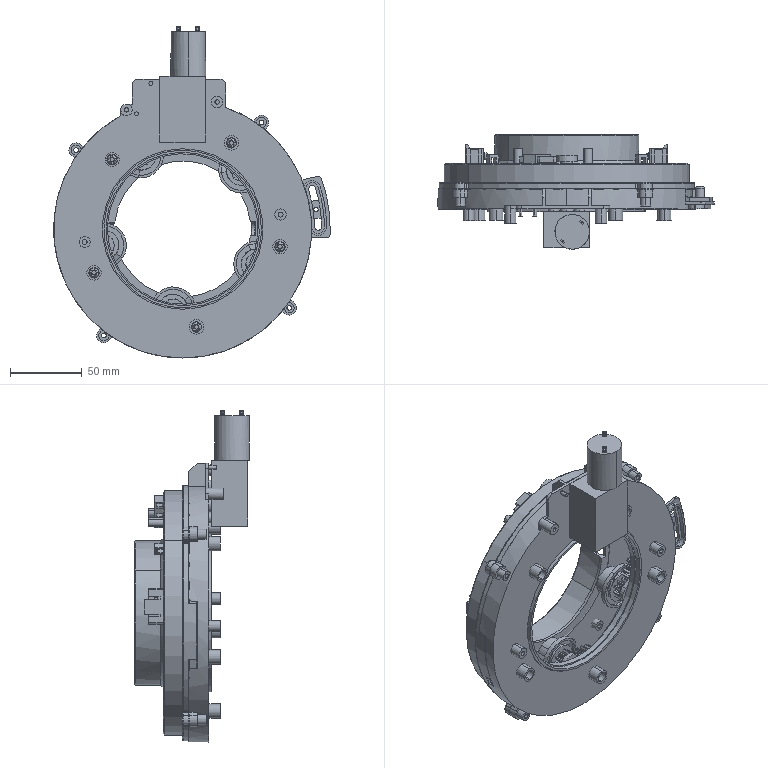Part | STEP file | 90-bore adjustable cup dropper with cup bucket assembly V1.201001 | 25 solids | 3175 faces | volume 341072 mm3 | plane 1690 | cylinder 1318 | cone 89 | spline 45 | torus 31 | sphere 2 | commonest cylinder face diameters 0.997 x183 168.2 x132 24 x115 30 x110 15 x60 9.5 x55